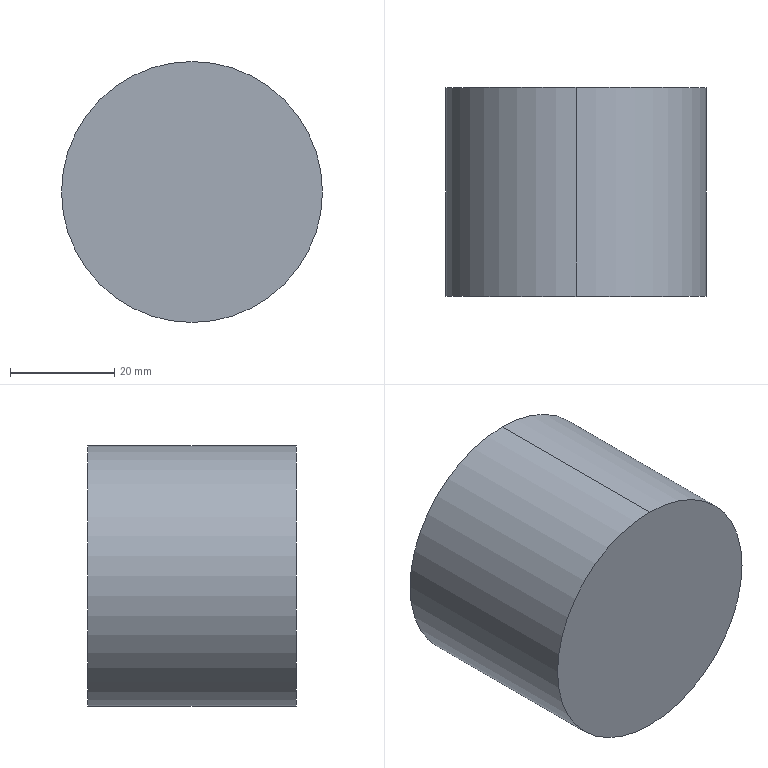Part | SolidWorks | features BaseBody 1 | 1 solid | 4 faces | box 50 x 40 x 50 mm | volume 78540 mm3 | plane 2 | cylinder 2 | commonest cylinder face diameters 50 x2
STEP:
#1=CARTESIAN_POINT('',(0.,0.,-25.));
#2=VERTEX_POINT('',#1);
#3=CARTESIAN_POINT('',(0.,0.,25.));
#4=VERTEX_POINT('',#3);
#5=CARTESIAN_POINT('',(0.,0.,0.));
#6=DIRECTION('',(0.,1.,0.));
#7=DIRECTION('',(0.,0.,1.));
#8=AXIS2_PLACEMENT_3D('',#5,#6,#7);
#9=CIRCLE('',#8,25.);
#10=EDGE_CURVE('',#2,#4,#9,.T.);
#11=ORIENTED_EDGE('',*,*,#10,.F.);
#12=CARTESIAN_POINT('',(0.,0.,0.));
#13=DIRECTION('',(0.,1.,0.));
#14=DIRECTION('',(0.,0.,1.));
#15=AXIS2_PLACEMENT_3D('',#12,#13,#14);
#16=CIRCLE('',#15,25.);
#17=EDGE_CURVE('',#4,#2,#16,.T.);
#18=ORIENTED_EDGE('',*,*,#17,.F.);
#19=EDGE_LOOP('',(#11,#18));
#20=FACE_OUTER_BOUND('',#19,.T.);
#21=CARTESIAN_POINT('',(0.,0.,0.));
#22=DIRECTION('',(0.,1.,0.));
#23=DIRECTION('',(1.,0.,0.));
#24=AXIS2_PLACEMENT_3D('',#21,#22,#23);
#25=PLANE('',#24);
#26=ADVANCED_FACE('',(#20),#25,.F.);
#27=CARTESIAN_POINT('',(0.,40.,-25.));
#28=VERTEX_POINT('',#27);
#29=CARTESIAN_POINT('',(0.,40.,25.));
#30=VERTEX_POINT('',#29);
#31=CARTESIAN_POINT('',(0.,40.,0.));
#32=DIRECTION('',(0.,1.,0.));
#33=DIRECTION('',(0.,0.,1.));
#34=AXIS2_PLACEMENT_3D('',#31,#32,#33);
#35=CIRCLE('',#34,25.);
#36=EDGE_CURVE('',#28,#30,#35,.T.);
#37=ORIENTED_EDGE('',*,*,#36,.T.);
#38=CARTESIAN_POINT('',(0.,40.,0.));
#39=DIRECTION('',(0.,1.,0.));
#40=DIRECTION('',(0.,0.,1.));
#41=AXIS2_PLACEMENT_3D('',#38,#39,#40);
#42=CIRCLE('',#41,25.);
#43=EDGE_CURVE('',#30,#28,#42,.T.);
#44=ORIENTED_EDGE('',*,*,#43,.T.);
#45=EDGE_LOOP('',(#37,#44));
#46=FACE_OUTER_BOUND('',#45,.T.);
#47=CARTESIAN_POINT('',(0.,40.,0.));
#48=DIRECTION('',(0.,1.,0.));
#49=DIRECTION('',(1.,0.,0.));
#50=AXIS2_PLACEMENT_3D('',#47,#48,#49);
#51=PLANE('',#50);
#52=ADVANCED_FACE('',(#46),#51,.T.);
#53=CARTESIAN_POINT('',(0.,40.,25.));
#54=DIRECTION('',(0.,-1.,0.));
#55=VECTOR('',#54,1000.);
#56=LINE('',#53,#55);
#57=EDGE_CURVE('',#30,#4,#56,.T.);
#58=ORIENTED_EDGE('',*,*,#57,.F.);
#59=ORIENTED_EDGE('',*,*,#36,.F.);
#60=CARTESIAN_POINT('',(0.,40.,-25.));
#61=DIRECTION('',(0.,-1.,0.));
#62=VECTOR('',#61,1000.);
#63=LINE('',#60,#62);
#64=EDGE_CURVE('',#28,#2,#63,.T.);
#65=ORIENTED_EDGE('',*,*,#64,.T.);
#66=ORIENTED_EDGE('',*,*,#10,.T.);
#67=EDGE_LOOP('',(#58,#59,#65,#66));
#68=FACE_OUTER_BOUND('',#67,.T.);
#69=CARTESIAN_POINT('',(0.,40.,0.));
#70=DIRECTION('',(0.,-1.,0.));
#71=DIRECTION('',(0.,0.,-1.));
#72=AXIS2_PLACEMENT_3D('',#69,#70,#71);
#73=CYLINDRICAL_SURFACE('',#72,25.);
#74=ADVANCED_FACE('',(#68),#73,.T.);
#75=ORIENTED_EDGE('',*,*,#43,.F.);
#76=ORIENTED_EDGE('',*,*,#57,.T.);
#77=ORIENTED_EDGE('',*,*,#17,.T.);
#78=ORIENTED_EDGE('',*,*,#64,.F.);
#79=EDGE_LOOP('',(#75,#76,#77,#78));
#80=FACE_OUTER_BOUND('',#79,.T.);
#81=CARTESIAN_POINT('',(0.,40.,0.));
#82=DIRECTION('',(0.,-1.,0.));
#83=DIRECTION('',(0.,0.,-1.));
#84=AXIS2_PLACEMENT_3D('',#81,#82,#83);
#85=CYLINDRICAL_SURFACE('',#84,25.);
#86=ADVANCED_FACE('',(#80),#85,.T.);
#87=CLOSED_SHELL('',(#26,#52,#74,#86));
#88=MANIFOLD_SOLID_BREP('',#87);
#89=CARTESIAN_POINT('',(0.,0.,0.));
#90=DIRECTION('',(0.,0.,1.));
#91=DIRECTION('',(1.,0.,0.));
#92=AXIS2_PLACEMENT_3D('',#89,#90,#91);
#93=(LENGTH_UNIT()NAMED_UNIT(*)SI_UNIT(.MILLI.,.METRE.));
#94=UNCERTAINTY_MEASURE_WITH_UNIT(LENGTH_MEASURE(0.00001),#93,'','');
#95=(NAMED_UNIT(*)PLANE_ANGLE_UNIT()SI_UNIT($,.RADIAN.));
#96=(NAMED_UNIT(*)SI_UNIT($,.STERADIAN.)SOLID_ANGLE_UNIT());
#97=(GEOMETRIC_REPRESENTATION_CONTEXT(3)GLOBAL_UNCERTAINTY_ASSIGNED_CONTEXT((#94))GLOBAL_UNIT_ASSIGNED_CONTEXT((#93,#95,#96))REPRESENTATION_CONTEXT('',''));
#98=ADVANCED_BREP_SHAPE_REPRESENTATION('',(#88,#92),#97);